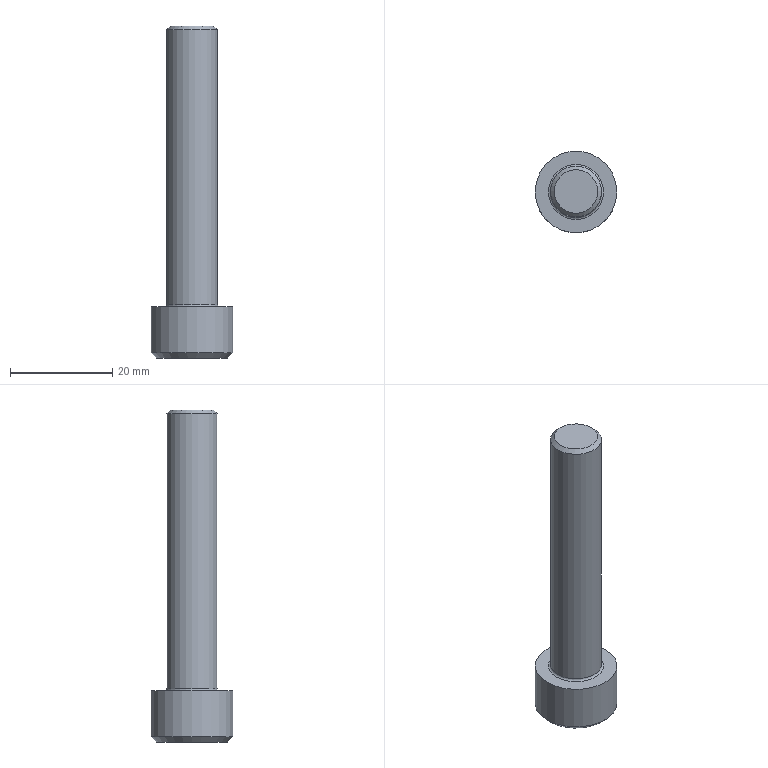Part | STEP file | solid 1 | 1 solid | 21 faces | box 16 x 16 x 65 mm | volume 6021 mm3 | plane 10 | sphere 6 | cylinder 2 | cone 2 | torus 1 | commonest cylinder face diameters 10 x1 16 x1